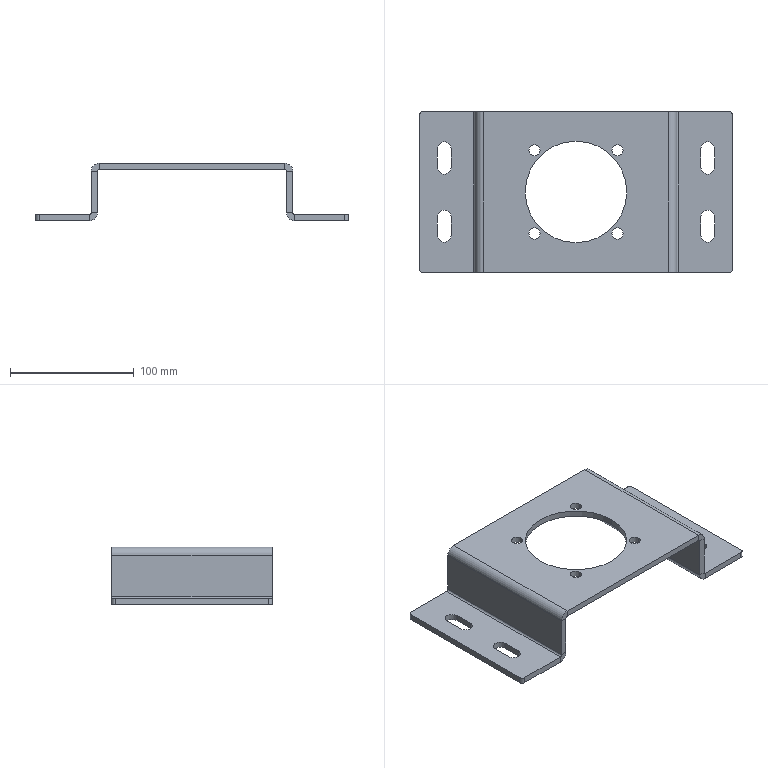Part | STEP file | 10-Roller motor plate | 1 solid | 68 faces | box 253 x 130 x 46.5 mm | volume 181020 mm3 | plane 38 | cylinder 30 | commonest cylinder face diameters 9 x8 11 x8 3 x4 6 x4 13 x4 82 x2